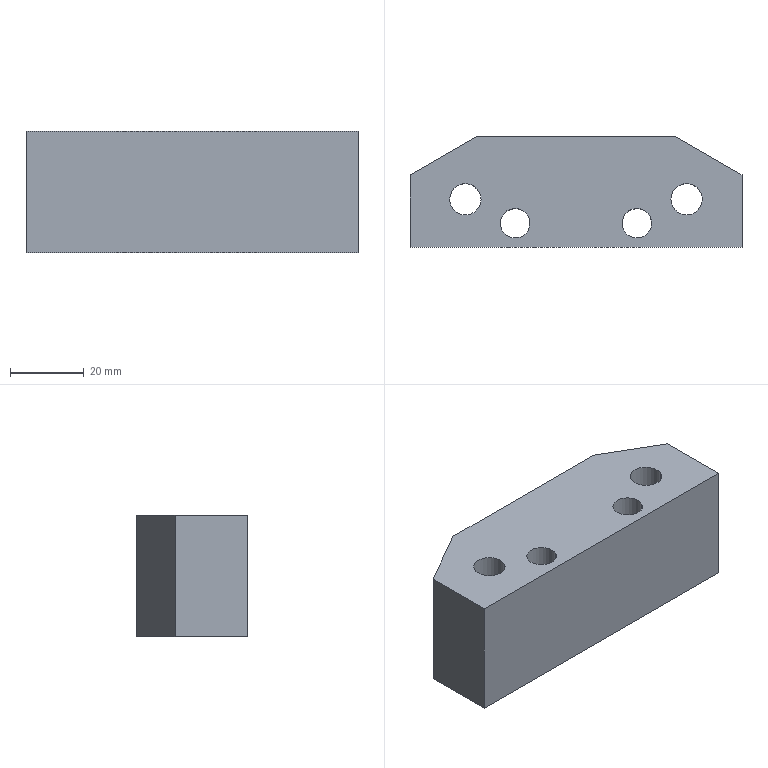Part | CATIA | 1 solid | 16 faces | box 90 x 30 x 33 mm | volume 75864 mm3 | plane 8 | cylinder 8 | commonest cylinder face diameters 8 x4 8.5 x4
STEP:
#1=CARTESIAN_POINT('',(45.,-30.,38.));
#2=VERTEX_POINT('',#1);
#3=CARTESIAN_POINT('',(45.,-30.,5.));
#4=VERTEX_POINT('',#3);
#5=CARTESIAN_POINT('',(45.,-30.,21.5));
#6=DIRECTION('',(0.,0.,-1.));
#7=VECTOR('',#6,1.);
#8=LINE('',#5,#7);
#9=EDGE_CURVE('',#2,#4,#8,.T.);
#10=ORIENTED_EDGE('',*,*,#9,.F.);
#11=CARTESIAN_POINT('',(-45.,-30.,38.));
#12=VERTEX_POINT('',#11);
#13=CARTESIAN_POINT('',(0.,-30.,38.));
#14=DIRECTION('',(-1.,0.,0.));
#15=VECTOR('',#14,1.);
#16=LINE('',#13,#15);
#17=EDGE_CURVE('',#2,#12,#16,.T.);
#18=ORIENTED_EDGE('',*,*,#17,.T.);
#19=CARTESIAN_POINT('',(-45.,-30.,5.));
#20=VERTEX_POINT('',#19);
#21=CARTESIAN_POINT('',(-45.,-30.,21.5));
#22=DIRECTION('',(0.,0.,-1.));
#23=VECTOR('',#22,1.);
#24=LINE('',#21,#23);
#25=EDGE_CURVE('',#12,#20,#24,.T.);
#26=ORIENTED_EDGE('',*,*,#25,.T.);
#27=CARTESIAN_POINT('',(0.,-30.,5.));
#28=DIRECTION('',(-1.,0.,0.));
#29=VECTOR('',#28,1.);
#30=LINE('',#27,#29);
#31=EDGE_CURVE('',#4,#20,#30,.T.);
#32=ORIENTED_EDGE('',*,*,#31,.F.);
#33=EDGE_LOOP('',(#10,#18,#26,#32));
#34=FACE_OUTER_BOUND('',#33,.T.);
#35=CARTESIAN_POINT('',(45.,-30.,38.));
#36=DIRECTION('',(0.,-1.,0.));
#37=DIRECTION('',(-1.,0.,0.));
#38=AXIS2_PLACEMENT_3D('',#35,#36,#37);
#39=PLANE('',#38);
#40=ADVANCED_FACE('',(#34),#39,.T.);
#41=CARTESIAN_POINT('',(-45.,-10.392,38.));
#42=VERTEX_POINT('',#41);
#43=CARTESIAN_POINT('',(-45.,-10.392,5.));
#44=VERTEX_POINT('',#43);
#45=CARTESIAN_POINT('',(-45.,-10.392,21.5));
#46=DIRECTION('',(0.,0.,-1.));
#47=VECTOR('',#46,1.);
#48=LINE('',#45,#47);
#49=EDGE_CURVE('',#42,#44,#48,.T.);
#50=ORIENTED_EDGE('',*,*,#49,.T.);
#51=CARTESIAN_POINT('',(-45.,-20.196,5.));
#52=DIRECTION('',(0.,-1.,0.));
#53=VECTOR('',#52,1.);
#54=LINE('',#51,#53);
#55=EDGE_CURVE('',#20,#44,#54,.F.);
#56=ORIENTED_EDGE('',*,*,#55,.F.);
#57=ORIENTED_EDGE('',*,*,#25,.F.);
#58=CARTESIAN_POINT('',(-45.,-20.196,38.));
#59=DIRECTION('',(0.,-1.,0.));
#60=VECTOR('',#59,1.);
#61=LINE('',#58,#60);
#62=EDGE_CURVE('',#12,#42,#61,.F.);
#63=ORIENTED_EDGE('',*,*,#62,.T.);
#64=EDGE_LOOP('',(#50,#56,#57,#63));
#65=FACE_OUTER_BOUND('',#64,.T.);
#66=CARTESIAN_POINT('',(-45.,0.,38.));
#67=DIRECTION('',(1.,0.,0.));
#68=DIRECTION('',(0.,-1.,0.));
#69=AXIS2_PLACEMENT_3D('',#66,#67,#68);
#70=PLANE('',#69);
#71=ADVANCED_FACE('',(#65),#70,.F.);
#72=CARTESIAN_POINT('',(-27.,0.,5.));
#73=VERTEX_POINT('',#72);
#74=CARTESIAN_POINT('',(-36.,-5.196,5.));
#75=DIRECTION('',(-0.866,-0.5,0.));
#76=VECTOR('',#75,1.);
#77=LINE('',#74,#76);
#78=EDGE_CURVE('',#73,#44,#77,.T.);
#79=ORIENTED_EDGE('',*,*,#78,.T.);
#80=ORIENTED_EDGE('',*,*,#49,.F.);
#81=CARTESIAN_POINT('',(-27.,0.,38.));
#82=VERTEX_POINT('',#81);
#83=CARTESIAN_POINT('',(-36.,-5.196,38.));
#84=DIRECTION('',(-0.866,-0.5,0.));
#85=VECTOR('',#84,1.);
#86=LINE('',#83,#85);
#87=EDGE_CURVE('',#42,#82,#86,.F.);
#88=ORIENTED_EDGE('',*,*,#87,.T.);
#89=CARTESIAN_POINT('',(-27.,0.,21.5));
#90=DIRECTION('',(0.,0.,-1.));
#91=VECTOR('',#90,1.);
#92=LINE('',#89,#91);
#93=EDGE_CURVE('',#82,#73,#92,.T.);
#94=ORIENTED_EDGE('',*,*,#93,.T.);
#95=EDGE_LOOP('',(#79,#80,#88,#94));
#96=FACE_OUTER_BOUND('',#95,.T.);
#97=CARTESIAN_POINT('',(-27.,0.,44.6));
#98=DIRECTION('',(-0.5,0.866,0.));
#99=DIRECTION('',(0.,0.,-1.));
#100=AXIS2_PLACEMENT_3D('',#97,#98,#99);
#101=PLANE('',#100);
#102=ADVANCED_FACE('',(#96),#101,.T.);
#103=CARTESIAN_POINT('',(45.,-10.392,38.));
#104=VERTEX_POINT('',#103);
#105=CARTESIAN_POINT('',(45.,-10.392,5.));
#106=VERTEX_POINT('',#105);
#107=CARTESIAN_POINT('',(45.,-10.392,21.5));
#108=DIRECTION('',(0.,0.,1.));
#109=VECTOR('',#108,1.);
#110=LINE('',#107,#109);
#111=EDGE_CURVE('',#104,#106,#110,.F.);
#112=ORIENTED_EDGE('',*,*,#111,.F.);
#113=CARTESIAN_POINT('',(45.,-20.196,38.));
#114=DIRECTION('',(0.,1.,0.));
#115=VECTOR('',#114,1.);
#116=LINE('',#113,#115);
#117=EDGE_CURVE('',#104,#2,#116,.F.);
#118=ORIENTED_EDGE('',*,*,#117,.T.);
#119=ORIENTED_EDGE('',*,*,#9,.T.);
#120=CARTESIAN_POINT('',(45.,-20.196,5.));
#121=DIRECTION('',(0.,1.,0.));
#122=VECTOR('',#121,1.);
#123=LINE('',#120,#122);
#124=EDGE_CURVE('',#106,#4,#123,.F.);
#125=ORIENTED_EDGE('',*,*,#124,.F.);
#126=EDGE_LOOP('',(#112,#118,#119,#125));
#127=FACE_OUTER_BOUND('',#126,.T.);
#128=CARTESIAN_POINT('',(45.,-30.,38.));
#129=DIRECTION('',(-1.,0.,0.));
#130=DIRECTION('',(0.,1.,0.));
#131=AXIS2_PLACEMENT_3D('',#128,#129,#130);
#132=PLANE('',#131);
#133=ADVANCED_FACE('',(#127),#132,.F.);
#134=CARTESIAN_POINT('',(27.,0.,5.));
#135=VERTEX_POINT('',#134);
#136=CARTESIAN_POINT('',(0.,0.,5.));
#137=DIRECTION('',(1.,0.,0.));
#138=VECTOR('',#137,1.);
#139=LINE('',#136,#138);
#140=EDGE_CURVE('',#73,#135,#139,.T.);
#141=ORIENTED_EDGE('',*,*,#140,.F.);
#142=ORIENTED_EDGE('',*,*,#93,.F.);
#143=CARTESIAN_POINT('',(27.,0.,38.));
#144=VERTEX_POINT('',#143);
#145=CARTESIAN_POINT('',(0.,0.,38.));
#146=DIRECTION('',(1.,0.,0.));
#147=VECTOR('',#146,1.);
#148=LINE('',#145,#147);
#149=EDGE_CURVE('',#82,#144,#148,.T.);
#150=ORIENTED_EDGE('',*,*,#149,.T.);
#151=CARTESIAN_POINT('',(27.,0.,21.5));
#152=DIRECTION('',(0.,0.,1.));
#153=VECTOR('',#152,1.);
#154=LINE('',#151,#153);
#155=EDGE_CURVE('',#144,#135,#154,.F.);
#156=ORIENTED_EDGE('',*,*,#155,.T.);
#157=EDGE_LOOP('',(#141,#142,#150,#156));
#158=FACE_OUTER_BOUND('',#157,.T.);
#159=CARTESIAN_POINT('',(-45.,0.,38.));
#160=DIRECTION('',(0.,1.,0.));
#161=DIRECTION('',(1.,0.,0.));
#162=AXIS2_PLACEMENT_3D('',#159,#160,#161);
#163=PLANE('',#162);
#164=ADVANCED_FACE('',(#158),#163,.T.);
#165=CARTESIAN_POINT('',(36.,-5.196,5.));
#166=DIRECTION('',(0.866,-0.5,0.));
#167=VECTOR('',#166,1.);
#168=LINE('',#165,#167);
#169=EDGE_CURVE('',#106,#135,#168,.F.);
#170=ORIENTED_EDGE('',*,*,#169,.T.);
#171=ORIENTED_EDGE('',*,*,#155,.F.);
#172=CARTESIAN_POINT('',(36.,-5.196,38.));
#173=DIRECTION('',(0.866,-0.5,0.));
#174=VECTOR('',#173,1.);
#175=LINE('',#172,#174);
#176=EDGE_CURVE('',#144,#104,#175,.T.);
#177=ORIENTED_EDGE('',*,*,#176,.T.);
#178=ORIENTED_EDGE('',*,*,#111,.T.);
#179=EDGE_LOOP('',(#170,#171,#177,#178));
#180=FACE_OUTER_BOUND('',#179,.T.);
#181=CARTESIAN_POINT('',(27.,0.,-1.6));
#182=DIRECTION('',(0.5,0.866,0.));
#183=DIRECTION('',(0.,0.,1.));
#184=AXIS2_PLACEMENT_3D('',#181,#182,#183);
#185=PLANE('',#184);
#186=ADVANCED_FACE('',(#180),#185,.T.);
#187=ORIENTED_EDGE('',*,*,#124,.T.);
#188=ORIENTED_EDGE('',*,*,#31,.T.);
#189=ORIENTED_EDGE('',*,*,#55,.T.);
#190=ORIENTED_EDGE('',*,*,#78,.F.);
#191=ORIENTED_EDGE('',*,*,#140,.T.);
#192=ORIENTED_EDGE('',*,*,#169,.F.);
#193=EDGE_LOOP('',(#187,#188,#189,#190,#191,#192));
#194=FACE_OUTER_BOUND('',#193,.T.);
#195=CARTESIAN_POINT('',(-33.73,-14.962,5.));
#196=VERTEX_POINT('',#195);
#197=CARTESIAN_POINT('',(-26.27,-19.038,5.));
#198=VERTEX_POINT('',#197);
#199=CARTESIAN_POINT('',(-30.,-17.,5.));
#200=DIRECTION('',(0.,0.,-1.));
#201=AXIS2_PLACEMENT_3D('',#199,#200,$);
#202=CIRCLE('',#201,4.25);
#203=EDGE_CURVE('',#196,#198,#202,.T.);
#204=ORIENTED_EDGE('',*,*,#203,.F.);
#205=CARTESIAN_POINT('',(-30.,-17.,5.));
#206=DIRECTION('',(0.,0.,-1.));
#207=AXIS2_PLACEMENT_3D('',#205,#206,$);
#208=CIRCLE('',#207,4.25);
#209=EDGE_CURVE('',#198,#196,#208,.T.);
#210=ORIENTED_EDGE('',*,*,#209,.F.);
#211=EDGE_LOOP('',(#204,#210));
#212=FACE_BOUND('',#211,.T.);
#213=CARTESIAN_POINT('',(26.27,-14.962,5.));
#214=VERTEX_POINT('',#213);
#215=CARTESIAN_POINT('',(33.73,-19.038,5.));
#216=VERTEX_POINT('',#215);
#217=CARTESIAN_POINT('',(30.,-17.,5.));
#218=DIRECTION('',(0.,0.,-1.));
#219=AXIS2_PLACEMENT_3D('',#217,#218,$);
#220=CIRCLE('',#219,4.25);
#221=EDGE_CURVE('',#214,#216,#220,.T.);
#222=ORIENTED_EDGE('',*,*,#221,.F.);
#223=CARTESIAN_POINT('',(30.,-17.,5.));
#224=DIRECTION('',(0.,0.,-1.));
#225=AXIS2_PLACEMENT_3D('',#223,#224,$);
#226=CIRCLE('',#225,4.25);
#227=EDGE_CURVE('',#216,#214,#226,.T.);
#228=ORIENTED_EDGE('',*,*,#227,.F.);
#229=EDGE_LOOP('',(#222,#228));
#230=FACE_BOUND('',#229,.T.);
#231=CARTESIAN_POINT('',(-20.01,-21.582,5.));
#232=VERTEX_POINT('',#231);
#233=CARTESIAN_POINT('',(-12.99,-25.418,5.));
#234=VERTEX_POINT('',#233);
#235=CARTESIAN_POINT('',(-16.5,-23.5,5.));
#236=DIRECTION('',(0.,0.,-1.));
#237=AXIS2_PLACEMENT_3D('',#235,#236,$);
#238=CIRCLE('',#237,4.);
#239=EDGE_CURVE('',#232,#234,#238,.T.);
#240=ORIENTED_EDGE('',*,*,#239,.F.);
#241=CARTESIAN_POINT('',(-16.5,-23.5,5.));
#242=DIRECTION('',(0.,0.,-1.));
#243=AXIS2_PLACEMENT_3D('',#241,#242,$);
#244=CIRCLE('',#243,4.);
#245=EDGE_CURVE('',#234,#232,#244,.T.);
#246=ORIENTED_EDGE('',*,*,#245,.F.);
#247=EDGE_LOOP('',(#240,#246));
#248=FACE_BOUND('',#247,.T.);
#249=CARTESIAN_POINT('',(12.99,-21.582,5.));
#250=VERTEX_POINT('',#249);
#251=CARTESIAN_POINT('',(20.01,-25.418,5.));
#252=VERTEX_POINT('',#251);
#253=CARTESIAN_POINT('',(16.5,-23.5,5.));
#254=DIRECTION('',(0.,0.,-1.));
#255=AXIS2_PLACEMENT_3D('',#253,#254,$);
#256=CIRCLE('',#255,4.);
#257=EDGE_CURVE('',#250,#252,#256,.T.);
#258=ORIENTED_EDGE('',*,*,#257,.F.);
#259=CARTESIAN_POINT('',(16.5,-23.5,5.));
#260=DIRECTION('',(0.,0.,-1.));
#261=AXIS2_PLACEMENT_3D('',#259,#260,$);
#262=CIRCLE('',#261,4.);
#263=EDGE_CURVE('',#252,#250,#262,.T.);
#264=ORIENTED_EDGE('',*,*,#263,.F.);
#265=EDGE_LOOP('',(#258,#264));
#266=FACE_BOUND('',#265,.T.);
#267=CARTESIAN_POINT('',(0.,0.,5.));
#268=DIRECTION('',(0.,0.,-1.));
#269=DIRECTION('',(1.,0.,0.));
#270=AXIS2_PLACEMENT_3D('',#267,#268,#269);
#271=PLANE('',#270);
#272=ADVANCED_FACE('',(#194,#212,#230,#248,#266),#271,.T.);
#273=ORIENTED_EDGE('',*,*,#176,.F.);
#274=ORIENTED_EDGE('',*,*,#149,.F.);
#275=ORIENTED_EDGE('',*,*,#87,.F.);
#276=ORIENTED_EDGE('',*,*,#62,.F.);
#277=ORIENTED_EDGE('',*,*,#17,.F.);
#278=ORIENTED_EDGE('',*,*,#117,.F.);
#279=EDGE_LOOP('',(#273,#274,#275,#276,#277,#278));
#280=FACE_OUTER_BOUND('',#279,.T.);
#281=CARTESIAN_POINT('',(-33.73,-14.962,38.));
#282=VERTEX_POINT('',#281);
#283=CARTESIAN_POINT('',(-26.27,-19.038,38.));
#284=VERTEX_POINT('',#283);
#285=CARTESIAN_POINT('',(-30.,-17.,38.));
#286=DIRECTION('',(0.,0.,-1.));
#287=AXIS2_PLACEMENT_3D('',#285,#286,$);
#288=CIRCLE('',#287,4.25);
#289=EDGE_CURVE('',#282,#284,#288,.T.);
#290=ORIENTED_EDGE('',*,*,#289,.T.);
#291=CARTESIAN_POINT('',(-30.,-17.,38.));
#292=DIRECTION('',(0.,0.,-1.));
#293=AXIS2_PLACEMENT_3D('',#291,#292,$);
#294=CIRCLE('',#293,4.25);
#295=EDGE_CURVE('',#284,#282,#294,.T.);
#296=ORIENTED_EDGE('',*,*,#295,.T.);
#297=EDGE_LOOP('',(#290,#296));
#298=FACE_BOUND('',#297,.T.);
#299=CARTESIAN_POINT('',(26.27,-14.962,38.));
#300=VERTEX_POINT('',#299);
#301=CARTESIAN_POINT('',(33.73,-19.038,38.));
#302=VERTEX_POINT('',#301);
#303=CARTESIAN_POINT('',(30.,-17.,38.));
#304=DIRECTION('',(0.,0.,-1.));
#305=AXIS2_PLACEMENT_3D('',#303,#304,$);
#306=CIRCLE('',#305,4.25);
#307=EDGE_CURVE('',#300,#302,#306,.T.);
#308=ORIENTED_EDGE('',*,*,#307,.T.);
#309=CARTESIAN_POINT('',(30.,-17.,38.));
#310=DIRECTION('',(0.,0.,-1.));
#311=AXIS2_PLACEMENT_3D('',#309,#310,$);
#312=CIRCLE('',#311,4.25);
#313=EDGE_CURVE('',#302,#300,#312,.T.);
#314=ORIENTED_EDGE('',*,*,#313,.T.);
#315=EDGE_LOOP('',(#308,#314));
#316=FACE_BOUND('',#315,.T.);
#317=CARTESIAN_POINT('',(-20.01,-21.582,38.));
#318=VERTEX_POINT('',#317);
#319=CARTESIAN_POINT('',(-12.99,-25.418,38.));
#320=VERTEX_POINT('',#319);
#321=CARTESIAN_POINT('',(-16.5,-23.5,38.));
#322=DIRECTION('',(0.,0.,-1.));
#323=AXIS2_PLACEMENT_3D('',#321,#322,$);
#324=CIRCLE('',#323,4.);
#325=EDGE_CURVE('',#318,#320,#324,.T.);
#326=ORIENTED_EDGE('',*,*,#325,.T.);
#327=CARTESIAN_POINT('',(-16.5,-23.5,38.));
#328=DIRECTION('',(0.,0.,-1.));
#329=AXIS2_PLACEMENT_3D('',#327,#328,$);
#330=CIRCLE('',#329,4.);
#331=EDGE_CURVE('',#320,#318,#330,.T.);
#332=ORIENTED_EDGE('',*,*,#331,.T.);
#333=EDGE_LOOP('',(#326,#332));
#334=FACE_BOUND('',#333,.T.);
#335=CARTESIAN_POINT('',(12.99,-21.582,38.));
#336=VERTEX_POINT('',#335);
#337=CARTESIAN_POINT('',(20.01,-25.418,38.));
#338=VERTEX_POINT('',#337);
#339=CARTESIAN_POINT('',(16.5,-23.5,38.));
#340=DIRECTION('',(0.,0.,-1.));
#341=AXIS2_PLACEMENT_3D('',#339,#340,$);
#342=CIRCLE('',#341,4.);
#343=EDGE_CURVE('',#336,#338,#342,.T.);
#344=ORIENTED_EDGE('',*,*,#343,.T.);
#345=CARTESIAN_POINT('',(16.5,-23.5,38.));
#346=DIRECTION('',(0.,0.,-1.));
#347=AXIS2_PLACEMENT_3D('',#345,#346,$);
#348=CIRCLE('',#347,4.);
#349=EDGE_CURVE('',#338,#336,#348,.T.);
#350=ORIENTED_EDGE('',*,*,#349,.T.);
#351=EDGE_LOOP('',(#344,#350));
#352=FACE_BOUND('',#351,.T.);
#353=CARTESIAN_POINT('',(0.,0.,38.));
#354=DIRECTION('',(0.,0.,-1.));
#355=DIRECTION('',(1.,0.,0.));
#356=AXIS2_PLACEMENT_3D('',#353,#354,#355);
#357=PLANE('',#356);
#358=ADVANCED_FACE('',(#280,#298,#316,#334,#352),#357,.F.);
#359=ORIENTED_EDGE('',*,*,#331,.F.);
#360=CARTESIAN_POINT('',(-12.99,-25.418,21.5));
#361=DIRECTION('',(0.,0.,-1.));
#362=VECTOR('',#361,1.);
#363=LINE('',#360,#362);
#364=EDGE_CURVE('',#234,#320,#363,.F.);
#365=ORIENTED_EDGE('',*,*,#364,.F.);
#366=ORIENTED_EDGE('',*,*,#245,.T.);
#367=CARTESIAN_POINT('',(-20.01,-21.582,21.5));
#368=DIRECTION('',(0.,0.,-1.));
#369=VECTOR('',#368,1.);
#370=LINE('',#367,#369);
#371=EDGE_CURVE('',#232,#318,#370,.F.);
#372=ORIENTED_EDGE('',*,*,#371,.T.);
#373=EDGE_LOOP('',(#359,#365,#366,#372));
#374=FACE_OUTER_BOUND('',#373,.T.);
#375=CARTESIAN_POINT('',(-16.5,-23.5,37.9));
#376=DIRECTION('',(0.,0.,-1.));
#377=DIRECTION('',(0.8776,-0.4794,0.));
#378=AXIS2_PLACEMENT_3D('',#375,#376,#377);
#379=CYLINDRICAL_SURFACE('',#378,4.);
#380=ADVANCED_FACE('',(#374),#379,.F.);
#381=ORIENTED_EDGE('',*,*,#325,.F.);
#382=ORIENTED_EDGE('',*,*,#371,.F.);
#383=ORIENTED_EDGE('',*,*,#239,.T.);
#384=ORIENTED_EDGE('',*,*,#364,.T.);
#385=EDGE_LOOP('',(#381,#382,#383,#384));
#386=FACE_OUTER_BOUND('',#385,.T.);
#387=ADVANCED_FACE('',(#386),#379,.F.);
#388=ORIENTED_EDGE('',*,*,#313,.F.);
#389=CARTESIAN_POINT('',(33.73,-19.038,21.5));
#390=DIRECTION('',(0.,0.,-1.));
#391=VECTOR('',#390,1.);
#392=LINE('',#389,#391);
#393=EDGE_CURVE('',#216,#302,#392,.F.);
#394=ORIENTED_EDGE('',*,*,#393,.F.);
#395=ORIENTED_EDGE('',*,*,#227,.T.);
#396=CARTESIAN_POINT('',(26.27,-14.962,21.5));
#397=DIRECTION('',(0.,0.,-1.));
#398=VECTOR('',#397,1.);
#399=LINE('',#396,#398);
#400=EDGE_CURVE('',#214,#300,#399,.F.);
#401=ORIENTED_EDGE('',*,*,#400,.T.);
#402=EDGE_LOOP('',(#388,#394,#395,#401));
#403=FACE_OUTER_BOUND('',#402,.T.);
#404=CARTESIAN_POINT('',(30.,-17.,37.9));
#405=DIRECTION('',(0.,0.,-1.));
#406=DIRECTION('',(0.8776,-0.4794,0.));
#407=AXIS2_PLACEMENT_3D('',#404,#405,#406);
#408=CYLINDRICAL_SURFACE('',#407,4.25);
#409=ADVANCED_FACE('',(#403),#408,.F.);
#410=ORIENTED_EDGE('',*,*,#307,.F.);
#411=ORIENTED_EDGE('',*,*,#400,.F.);
#412=ORIENTED_EDGE('',*,*,#221,.T.);
#413=ORIENTED_EDGE('',*,*,#393,.T.);
#414=EDGE_LOOP('',(#410,#411,#412,#413));
#415=FACE_OUTER_BOUND('',#414,.T.);
#416=ADVANCED_FACE('',(#415),#408,.F.);
#417=ORIENTED_EDGE('',*,*,#349,.F.);
#418=CARTESIAN_POINT('',(20.01,-25.418,21.5));
#419=DIRECTION('',(0.,0.,-1.));
#420=VECTOR('',#419,1.);
#421=LINE('',#418,#420);
#422=EDGE_CURVE('',#252,#338,#421,.F.);
#423=ORIENTED_EDGE('',*,*,#422,.F.);
#424=ORIENTED_EDGE('',*,*,#263,.T.);
#425=CARTESIAN_POINT('',(12.99,-21.582,21.5));
#426=DIRECTION('',(0.,0.,-1.));
#427=VECTOR('',#426,1.);
#428=LINE('',#425,#427);
#429=EDGE_CURVE('',#250,#336,#428,.F.);
#430=ORIENTED_EDGE('',*,*,#429,.T.);
#431=EDGE_LOOP('',(#417,#423,#424,#430));
#432=FACE_OUTER_BOUND('',#431,.T.);
#433=CARTESIAN_POINT('',(16.5,-23.5,37.9));
#434=DIRECTION('',(0.,0.,-1.));
#435=DIRECTION('',(0.8776,-0.4794,0.));
#436=AXIS2_PLACEMENT_3D('',#433,#434,#435);
#437=CYLINDRICAL_SURFACE('',#436,4.);
#438=ADVANCED_FACE('',(#432),#437,.F.);
#439=ORIENTED_EDGE('',*,*,#343,.F.);
#440=ORIENTED_EDGE('',*,*,#429,.F.);
#441=ORIENTED_EDGE('',*,*,#257,.T.);
#442=ORIENTED_EDGE('',*,*,#422,.T.);
#443=EDGE_LOOP('',(#439,#440,#441,#442));
#444=FACE_OUTER_BOUND('',#443,.T.);
#445=ADVANCED_FACE('',(#444),#437,.F.);
#446=ORIENTED_EDGE('',*,*,#295,.F.);
#447=CARTESIAN_POINT('',(-26.27,-19.038,21.5));
#448=DIRECTION('',(0.,0.,-1.));
#449=VECTOR('',#448,1.);
#450=LINE('',#447,#449);
#451=EDGE_CURVE('',#198,#284,#450,.F.);
#452=ORIENTED_EDGE('',*,*,#451,.F.);
#453=ORIENTED_EDGE('',*,*,#209,.T.);
#454=CARTESIAN_POINT('',(-33.73,-14.962,21.5));
#455=DIRECTION('',(0.,0.,-1.));
#456=VECTOR('',#455,1.);
#457=LINE('',#454,#456);
#458=EDGE_CURVE('',#196,#282,#457,.F.);
#459=ORIENTED_EDGE('',*,*,#458,.T.);
#460=EDGE_LOOP('',(#446,#452,#453,#459));
#461=FACE_OUTER_BOUND('',#460,.T.);
#462=CARTESIAN_POINT('',(-30.,-17.,37.9));
#463=DIRECTION('',(0.,0.,-1.));
#464=DIRECTION('',(0.8776,-0.4794,0.));
#465=AXIS2_PLACEMENT_3D('',#462,#463,#464);
#466=CYLINDRICAL_SURFACE('',#465,4.25);
#467=ADVANCED_FACE('',(#461),#466,.F.);
#468=ORIENTED_EDGE('',*,*,#289,.F.);
#469=ORIENTED_EDGE('',*,*,#458,.F.);
#470=ORIENTED_EDGE('',*,*,#203,.T.);
#471=ORIENTED_EDGE('',*,*,#451,.T.);
#472=EDGE_LOOP('',(#468,#469,#470,#471));
#473=FACE_OUTER_BOUND('',#472,.T.);
#474=ADVANCED_FACE('',(#473),#466,.F.);
#475=CLOSED_SHELL('',(#40,#71,#102,#133,#164,#186,#272,#358,#380,#387,#409,#416,#438,#445,#467,#474));
#476=MANIFOLD_SOLID_BREP('',#475);
#477=(LENGTH_UNIT()NAMED_UNIT(*)SI_UNIT(.MILLI.,.METRE.));
#478=UNCERTAINTY_MEASURE_WITH_UNIT(LENGTH_MEASURE(0.005),#477,'','');
#479=(NAMED_UNIT(*)PLANE_ANGLE_UNIT()SI_UNIT($,.RADIAN.));
#480=(NAMED_UNIT(*)SI_UNIT($,.STERADIAN.)SOLID_ANGLE_UNIT());
#481=(GEOMETRIC_REPRESENTATION_CONTEXT(3)GLOBAL_UNCERTAINTY_ASSIGNED_CONTEXT((#478))GLOBAL_UNIT_ASSIGNED_CONTEXT((#477,#479,#480))REPRESENTATION_CONTEXT('',''));
#482=ADVANCED_BREP_SHAPE_REPRESENTATION('',(#476),#481);